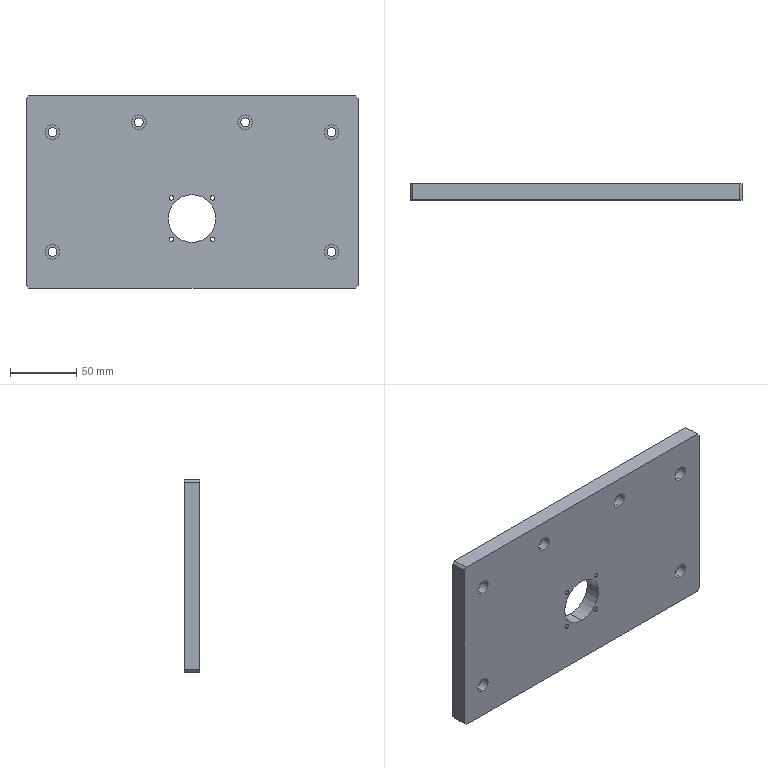Part | SolidWorks | features Cut 2, HoleWzd 2, Chamfer 1, Extrusion 1 | 1 solid | 62 faces | box 250 x 12 x 145 mm | volume 416706 mm3 | cylinder 42 | plane 20 | commonest cylinder face diameters 6.6 x12 11 x12 3.3 x8 10 x8 36 x2